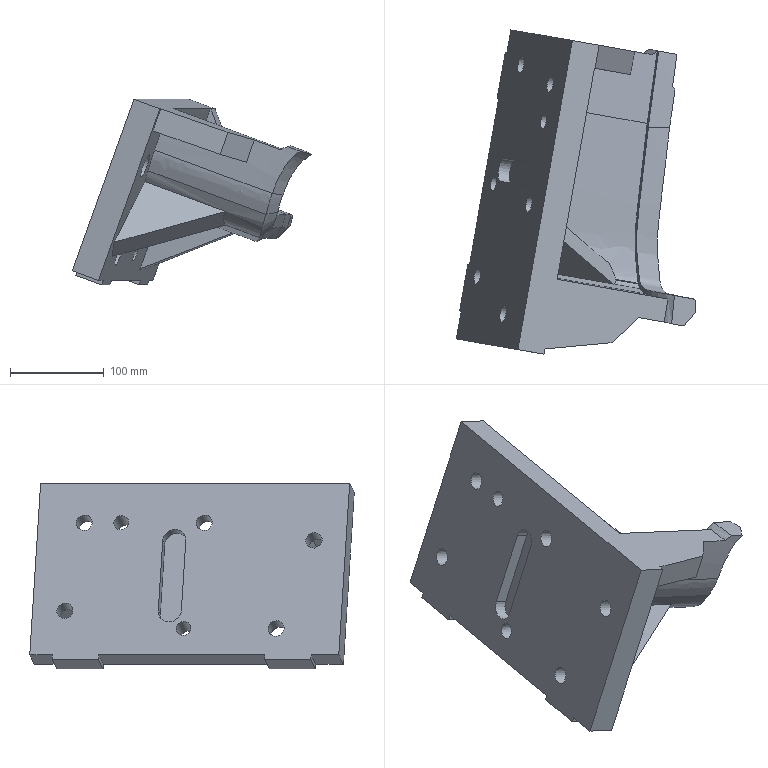Part | NX | features solid 2 | 1 solid | 85 faces | box 255.221 x 346.045 x 198.129 mm | volume 3492220 mm3 | plane 40 | spline 31 | cylinder 14 | commonest cylinder face diameters 25 x7 17.5 x5 16 x2